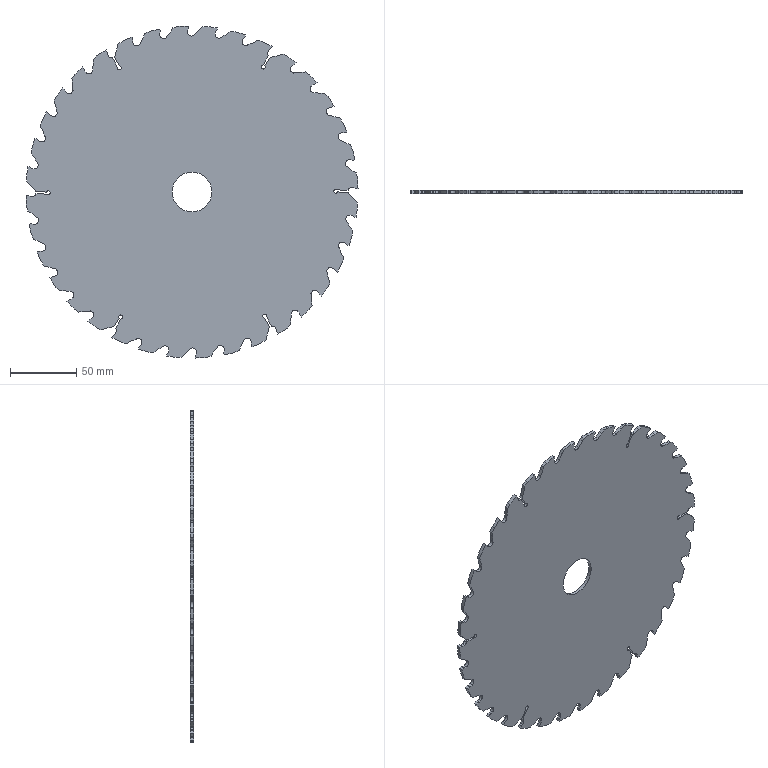Part | STEP file | DEWALT-DWE7492-B22 | 1 solid | 315 faces | box 249.95 x 2.5 x 249.95 mm | volume 115629 mm3 | plane 230 | cylinder 85 | commonest cylinder face diameters 5.6 x42 250 x36 3 x6 30 x1